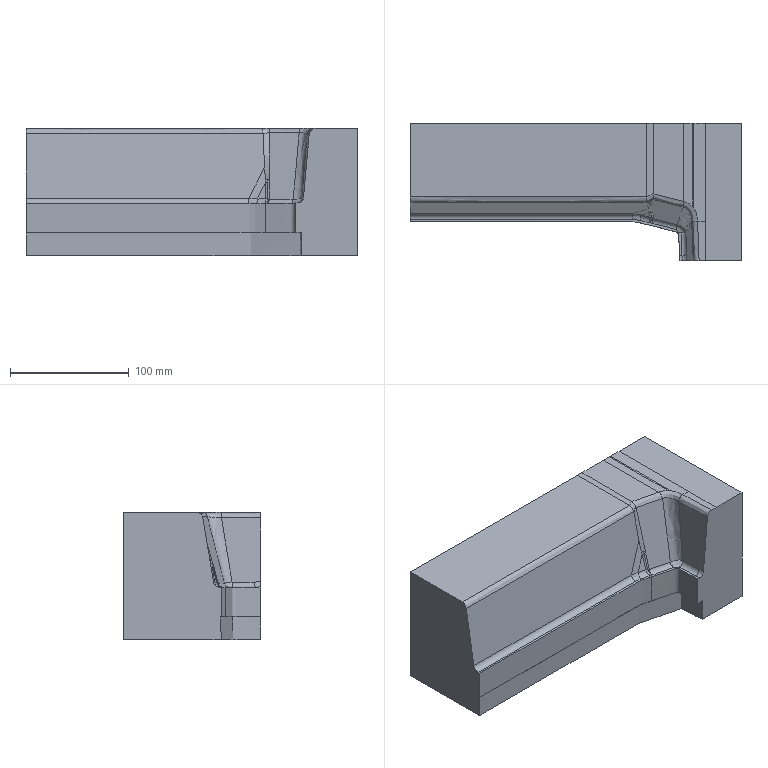Part | NX | features solid 2 | 1 solid | 55 faces | box 280 x 116 x 107.135 mm | volume 2471455 mm3 | spline 25 | plane 15 | cylinder 12 | cone 3 | commonest cylinder face diameters 12 x3 9 x2 10 x2 20 x2 8 x1 8.85 x1